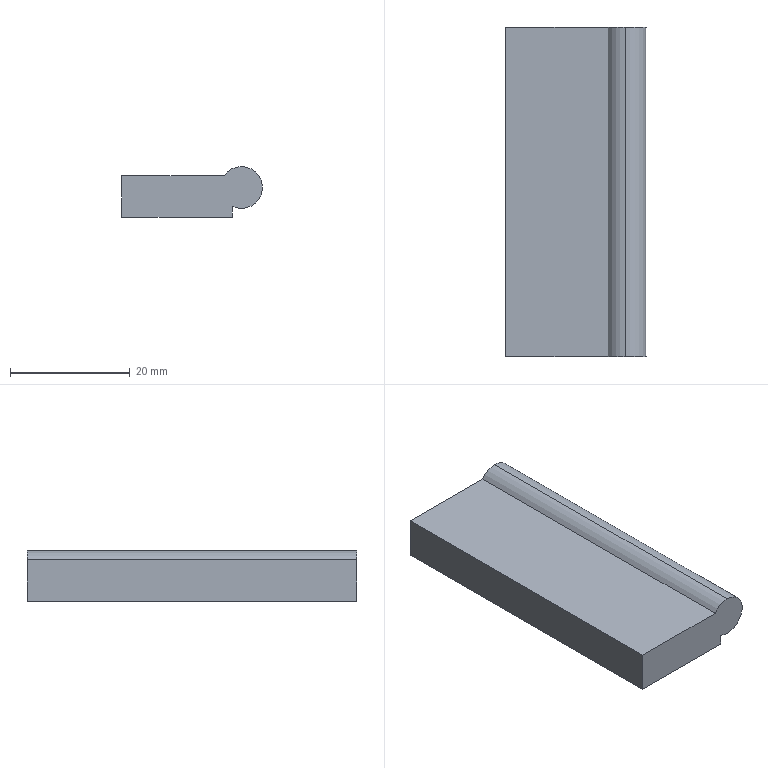Part | SolidWorks | features Extrusion 1, ICE 1 | 1 solid | 9 faces | box 23.5 x 55 x 8.5 mm | volume 8792 mm3 | plane 6 | cylinder 3 | commonest cylinder face diameters 7 x3
STEP:
#1=CARTESIAN_POINT('',(20.,0.,1.5));
#2=VERTEX_POINT('',#1);
#3=CARTESIAN_POINT('',(20.,0.,8.5));
#4=VERTEX_POINT('',#3);
#5=CARTESIAN_POINT('',(20.,0.,5.));
#6=DIRECTION('',(0.,-1.,0.));
#7=DIRECTION('',(0.,0.,1.));
#8=AXIS2_PLACEMENT_3D('',#5,#6,#7);
#9=CIRCLE('',#8,3.5);
#10=EDGE_CURVE('',#2,#4,#9,.T.);
#11=ORIENTED_EDGE('',*,*,#10,.F.);
#12=CARTESIAN_POINT('',(20.,55.,1.5));
#13=VERTEX_POINT('',#12);
#14=CARTESIAN_POINT('',(20.,-9.899,1.5));
#15=DIRECTION('',(0.,1.,0.));
#16=VECTOR('',#15,1000.);
#17=LINE('',#14,#16);
#18=EDGE_CURVE('',#2,#13,#17,.T.);
#19=ORIENTED_EDGE('',*,*,#18,.T.);
#20=CARTESIAN_POINT('',(20.,55.,8.5));
#21=VERTEX_POINT('',#20);
#22=CARTESIAN_POINT('',(20.,55.,5.));
#23=DIRECTION('',(0.,1.,0.));
#24=DIRECTION('',(0.,0.,1.));
#25=AXIS2_PLACEMENT_3D('',#22,#23,#24);
#26=CIRCLE('',#25,3.5);
#27=EDGE_CURVE('',#21,#13,#26,.T.);
#28=ORIENTED_EDGE('',*,*,#27,.F.);
#29=CARTESIAN_POINT('',(20.,-9.899,8.5));
#30=DIRECTION('',(0.,1.,0.));
#31=VECTOR('',#30,1000.);
#32=LINE('',#29,#31);
#33=EDGE_CURVE('',#4,#21,#32,.T.);
#34=ORIENTED_EDGE('',*,*,#33,.F.);
#35=EDGE_LOOP('',(#11,#19,#28,#34));
#36=FACE_OUTER_BOUND('',#35,.T.);
#37=CARTESIAN_POINT('',(20.,-9.899,5.));
#38=DIRECTION('',(0.,1.,0.));
#39=DIRECTION('',(0.,0.,1.));
#40=AXIS2_PLACEMENT_3D('',#37,#38,#39);
#41=CYLINDRICAL_SURFACE('',#40,3.5);
#42=ADVANCED_FACE('',(#36),#41,.T.);
#43=CARTESIAN_POINT('',(17.128,0.,7.));
#44=VERTEX_POINT('',#43);
#45=CARTESIAN_POINT('',(20.,0.,5.));
#46=DIRECTION('',(0.,-1.,0.));
#47=DIRECTION('',(0.,0.,1.));
#48=AXIS2_PLACEMENT_3D('',#45,#46,#47);
#49=CIRCLE('',#48,3.5);
#50=EDGE_CURVE('',#4,#44,#49,.T.);
#51=ORIENTED_EDGE('',*,*,#50,.F.);
#52=ORIENTED_EDGE('',*,*,#33,.T.);
#53=CARTESIAN_POINT('',(17.128,55.,7.));
#54=VERTEX_POINT('',#53);
#55=CARTESIAN_POINT('',(20.,55.,5.));
#56=DIRECTION('',(0.,1.,0.));
#57=DIRECTION('',(0.,0.,1.));
#58=AXIS2_PLACEMENT_3D('',#55,#56,#57);
#59=CIRCLE('',#58,3.5);
#60=EDGE_CURVE('',#54,#21,#59,.T.);
#61=ORIENTED_EDGE('',*,*,#60,.F.);
#62=CARTESIAN_POINT('',(17.128,-9.899,7.));
#63=DIRECTION('',(0.,1.,0.));
#64=VECTOR('',#63,1000.);
#65=LINE('',#62,#64);
#66=EDGE_CURVE('',#44,#54,#65,.T.);
#67=ORIENTED_EDGE('',*,*,#66,.F.);
#68=EDGE_LOOP('',(#51,#52,#61,#67));
#69=FACE_OUTER_BOUND('',#68,.T.);
#70=CARTESIAN_POINT('',(20.,-9.899,5.));
#71=DIRECTION('',(0.,1.,0.));
#72=DIRECTION('',(0.,0.,1.));
#73=AXIS2_PLACEMENT_3D('',#70,#71,#72);
#74=CYLINDRICAL_SURFACE('',#73,3.5);
#75=ADVANCED_FACE('',(#69),#74,.T.);
#76=CARTESIAN_POINT('',(0.,55.,0.));
#77=VERTEX_POINT('',#76);
#78=CARTESIAN_POINT('',(0.,0.,0.));
#79=VERTEX_POINT('',#78);
#80=CARTESIAN_POINT('',(0.,0.,0.));
#81=DIRECTION('',(0.,-1.,0.));
#82=VECTOR('',#81,1000.);
#83=LINE('',#80,#82);
#84=EDGE_CURVE('',#77,#79,#83,.T.);
#85=ORIENTED_EDGE('',*,*,#84,.T.);
#86=CARTESIAN_POINT('',(0.,0.,7.));
#87=VERTEX_POINT('',#86);
#88=CARTESIAN_POINT('',(0.,0.,7.));
#89=DIRECTION('',(0.,0.,-1.));
#90=VECTOR('',#89,1000.);
#91=LINE('',#88,#90);
#92=EDGE_CURVE('',#87,#79,#91,.T.);
#93=ORIENTED_EDGE('',*,*,#92,.F.);
#94=CARTESIAN_POINT('',(0.,55.,7.));
#95=VERTEX_POINT('',#94);
#96=CARTESIAN_POINT('',(0.,0.,7.));
#97=DIRECTION('',(0.,-1.,0.));
#98=VECTOR('',#97,1000.);
#99=LINE('',#96,#98);
#100=EDGE_CURVE('',#95,#87,#99,.T.);
#101=ORIENTED_EDGE('',*,*,#100,.F.);
#102=CARTESIAN_POINT('',(0.,55.,7.));
#103=DIRECTION('',(0.,0.,-1.));
#104=VECTOR('',#103,1000.);
#105=LINE('',#102,#104);
#106=EDGE_CURVE('',#95,#77,#105,.T.);
#107=ORIENTED_EDGE('',*,*,#106,.T.);
#108=EDGE_LOOP('',(#85,#93,#101,#107));
#109=FACE_OUTER_BOUND('',#108,.T.);
#110=CARTESIAN_POINT('',(0.,0.,7.));
#111=DIRECTION('',(1.,0.,0.));
#112=DIRECTION('',(0.,0.,-1.));
#113=AXIS2_PLACEMENT_3D('',#110,#111,#112);
#114=PLANE('',#113);
#115=ADVANCED_FACE('',(#109),#114,.F.);
#116=CARTESIAN_POINT('',(18.5,0.,1.838));
#117=VERTEX_POINT('',#116);
#118=CARTESIAN_POINT('',(18.5,0.,0.));
#119=VERTEX_POINT('',#118);
#120=CARTESIAN_POINT('',(18.5,0.,7.));
#121=DIRECTION('',(0.,0.,-1.));
#122=VECTOR('',#121,1000.);
#123=LINE('',#120,#122);
#124=EDGE_CURVE('',#117,#119,#123,.T.);
#125=ORIENTED_EDGE('',*,*,#124,.F.);
#126=CARTESIAN_POINT('',(20.,0.,5.));
#127=DIRECTION('',(0.,-1.,0.));
#128=DIRECTION('',(0.,0.,1.));
#129=AXIS2_PLACEMENT_3D('',#126,#127,#128);
#130=CIRCLE('',#129,3.5);
#131=EDGE_CURVE('',#117,#2,#130,.T.);
#132=ORIENTED_EDGE('',*,*,#131,.T.);
#133=ORIENTED_EDGE('',*,*,#10,.T.);
#134=ORIENTED_EDGE('',*,*,#50,.T.);
#135=CARTESIAN_POINT('',(0.,0.,7.));
#136=DIRECTION('',(1.,0.,0.));
#137=VECTOR('',#136,1000.);
#138=LINE('',#135,#137);
#139=EDGE_CURVE('',#87,#44,#138,.T.);
#140=ORIENTED_EDGE('',*,*,#139,.F.);
#141=ORIENTED_EDGE('',*,*,#92,.T.);
#142=CARTESIAN_POINT('',(0.,0.,0.));
#143=DIRECTION('',(1.,0.,0.));
#144=VECTOR('',#143,1000.);
#145=LINE('',#142,#144);
#146=EDGE_CURVE('',#79,#119,#145,.T.);
#147=ORIENTED_EDGE('',*,*,#146,.T.);
#148=EDGE_LOOP('',(#125,#132,#133,#134,#140,#141,#147));
#149=FACE_OUTER_BOUND('',#148,.T.);
#150=CARTESIAN_POINT('',(0.,0.,7.));
#151=DIRECTION('',(0.,1.,0.));
#152=DIRECTION('',(0.,0.,1.));
#153=AXIS2_PLACEMENT_3D('',#150,#151,#152);
#154=PLANE('',#153);
#155=ADVANCED_FACE('',(#149),#154,.F.);
#156=CARTESIAN_POINT('',(18.5,55.,1.838));
#157=VERTEX_POINT('',#156);
#158=CARTESIAN_POINT('',(18.5,55.,0.));
#159=VERTEX_POINT('',#158);
#160=CARTESIAN_POINT('',(18.5,55.,7.));
#161=DIRECTION('',(0.,0.,-1.));
#162=VECTOR('',#161,1000.);
#163=LINE('',#160,#162);
#164=EDGE_CURVE('',#157,#159,#163,.T.);
#165=ORIENTED_EDGE('',*,*,#164,.F.);
#166=CARTESIAN_POINT('',(18.5,-9.899,1.838));
#167=DIRECTION('',(0.,-1.,0.));
#168=VECTOR('',#167,1000.);
#169=LINE('',#166,#168);
#170=EDGE_CURVE('',#157,#117,#169,.T.);
#171=ORIENTED_EDGE('',*,*,#170,.T.);
#172=ORIENTED_EDGE('',*,*,#124,.T.);
#173=CARTESIAN_POINT('',(18.5,0.,0.));
#174=DIRECTION('',(0.,1.,0.));
#175=VECTOR('',#174,1000.);
#176=LINE('',#173,#175);
#177=EDGE_CURVE('',#119,#159,#176,.T.);
#178=ORIENTED_EDGE('',*,*,#177,.T.);
#179=EDGE_LOOP('',(#165,#171,#172,#178));
#180=FACE_OUTER_BOUND('',#179,.T.);
#181=CARTESIAN_POINT('',(18.5,0.,7.));
#182=DIRECTION('',(-1.,0.,0.));
#183=DIRECTION('',(0.,0.,1.));
#184=AXIS2_PLACEMENT_3D('',#181,#182,#183);
#185=PLANE('',#184);
#186=ADVANCED_FACE('',(#180),#185,.F.);
#187=ORIENTED_EDGE('',*,*,#60,.T.);
#188=ORIENTED_EDGE('',*,*,#27,.T.);
#189=CARTESIAN_POINT('',(20.,55.,5.));
#190=DIRECTION('',(0.,1.,0.));
#191=DIRECTION('',(0.,0.,1.));
#192=AXIS2_PLACEMENT_3D('',#189,#190,#191);
#193=CIRCLE('',#192,3.5);
#194=EDGE_CURVE('',#13,#157,#193,.T.);
#195=ORIENTED_EDGE('',*,*,#194,.T.);
#196=ORIENTED_EDGE('',*,*,#164,.T.);
#197=CARTESIAN_POINT('',(0.,55.,0.));
#198=DIRECTION('',(-1.,0.,0.));
#199=VECTOR('',#198,1000.);
#200=LINE('',#197,#199);
#201=EDGE_CURVE('',#159,#77,#200,.T.);
#202=ORIENTED_EDGE('',*,*,#201,.T.);
#203=ORIENTED_EDGE('',*,*,#106,.F.);
#204=CARTESIAN_POINT('',(0.,55.,7.));
#205=DIRECTION('',(-1.,0.,0.));
#206=VECTOR('',#205,1000.);
#207=LINE('',#204,#206);
#208=EDGE_CURVE('',#54,#95,#207,.T.);
#209=ORIENTED_EDGE('',*,*,#208,.F.);
#210=EDGE_LOOP('',(#187,#188,#195,#196,#202,#203,#209));
#211=FACE_OUTER_BOUND('',#210,.T.);
#212=CARTESIAN_POINT('',(0.,55.,7.));
#213=DIRECTION('',(0.,-1.,0.));
#214=DIRECTION('',(0.,0.,-1.));
#215=AXIS2_PLACEMENT_3D('',#212,#213,#214);
#216=PLANE('',#215);
#217=ADVANCED_FACE('',(#211),#216,.F.);
#218=ORIENTED_EDGE('',*,*,#139,.T.);
#219=ORIENTED_EDGE('',*,*,#66,.T.);
#220=ORIENTED_EDGE('',*,*,#208,.T.);
#221=ORIENTED_EDGE('',*,*,#100,.T.);
#222=EDGE_LOOP('',(#218,#219,#220,#221));
#223=FACE_OUTER_BOUND('',#222,.T.);
#224=CARTESIAN_POINT('',(0.,55.,7.));
#225=DIRECTION('',(0.,0.,-1.));
#226=DIRECTION('',(-1.,0.,0.));
#227=AXIS2_PLACEMENT_3D('',#224,#225,#226);
#228=PLANE('',#227);
#229=ADVANCED_FACE('',(#223),#228,.F.);
#230=ORIENTED_EDGE('',*,*,#84,.F.);
#231=ORIENTED_EDGE('',*,*,#201,.F.);
#232=ORIENTED_EDGE('',*,*,#177,.F.);
#233=ORIENTED_EDGE('',*,*,#146,.F.);
#234=EDGE_LOOP('',(#230,#231,#232,#233));
#235=FACE_OUTER_BOUND('',#234,.T.);
#236=CARTESIAN_POINT('',(0.,55.,0.));
#237=DIRECTION('',(0.,0.,-1.));
#238=DIRECTION('',(-1.,0.,0.));
#239=AXIS2_PLACEMENT_3D('',#236,#237,#238);
#240=PLANE('',#239);
#241=ADVANCED_FACE('',(#235),#240,.T.);
#242=ORIENTED_EDGE('',*,*,#18,.F.);
#243=ORIENTED_EDGE('',*,*,#131,.F.);
#244=ORIENTED_EDGE('',*,*,#170,.F.);
#245=ORIENTED_EDGE('',*,*,#194,.F.);
#246=EDGE_LOOP('',(#242,#243,#244,#245));
#247=FACE_OUTER_BOUND('',#246,.T.);
#248=CARTESIAN_POINT('',(20.,-9.899,5.));
#249=DIRECTION('',(0.,1.,0.));
#250=DIRECTION('',(0.,0.,1.));
#251=AXIS2_PLACEMENT_3D('',#248,#249,#250);
#252=CYLINDRICAL_SURFACE('',#251,3.5);
#253=ADVANCED_FACE('',(#247),#252,.T.);
#254=CLOSED_SHELL('',(#42,#75,#115,#155,#186,#217,#229,#241,#253));
#255=MANIFOLD_SOLID_BREP('',#254);
#256=CARTESIAN_POINT('',(0.,0.,0.));
#257=DIRECTION('',(0.,0.,1.));
#258=DIRECTION('',(1.,0.,0.));
#259=AXIS2_PLACEMENT_3D('',#256,#257,#258);
#260=(LENGTH_UNIT()NAMED_UNIT(*)SI_UNIT(.MILLI.,.METRE.));
#261=UNCERTAINTY_MEASURE_WITH_UNIT(LENGTH_MEASURE(0.00001),#260,'','');
#262=(NAMED_UNIT(*)PLANE_ANGLE_UNIT()SI_UNIT($,.RADIAN.));
#263=(NAMED_UNIT(*)SI_UNIT($,.STERADIAN.)SOLID_ANGLE_UNIT());
#264=(GEOMETRIC_REPRESENTATION_CONTEXT(3)GLOBAL_UNCERTAINTY_ASSIGNED_CONTEXT((#261))GLOBAL_UNIT_ASSIGNED_CONTEXT((#260,#262,#263))REPRESENTATION_CONTEXT('',''));
#265=ADVANCED_BREP_SHAPE_REPRESENTATION('',(#255,#259),#264);